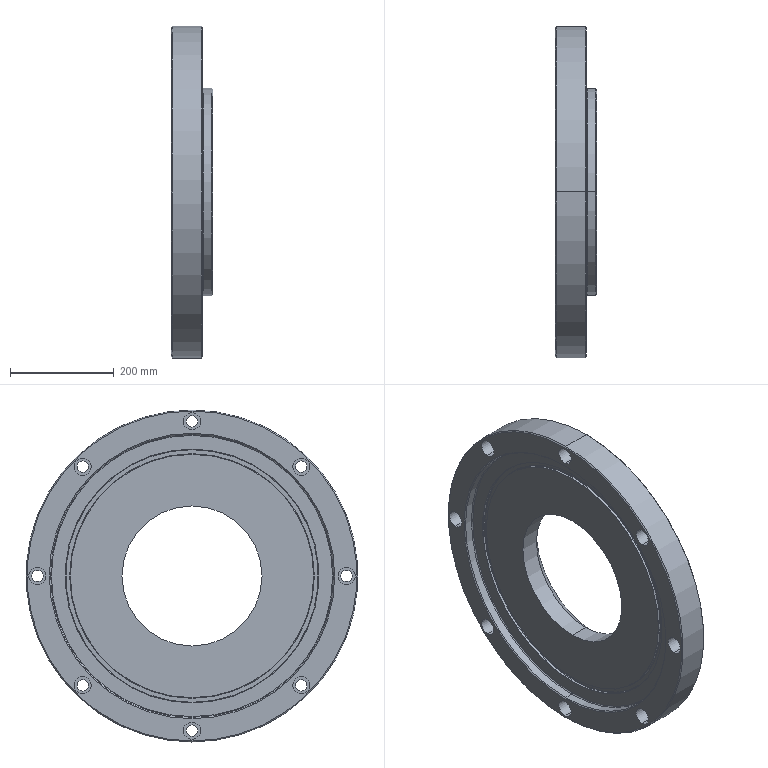Part | SolidWorks | features Chamfer 2, Fillet 2, ICE 2, Revolution 1 | 1 solid | 97 faces | box 80 x 640 x 640 mm | volume 12908044 mm3 | cylinder 48 | torus 20 | plane 17 | cone 12 | commonest cylinder face diameters 22 x16 33 x16 270 x2 400 x2 419.6 x2 439 x2